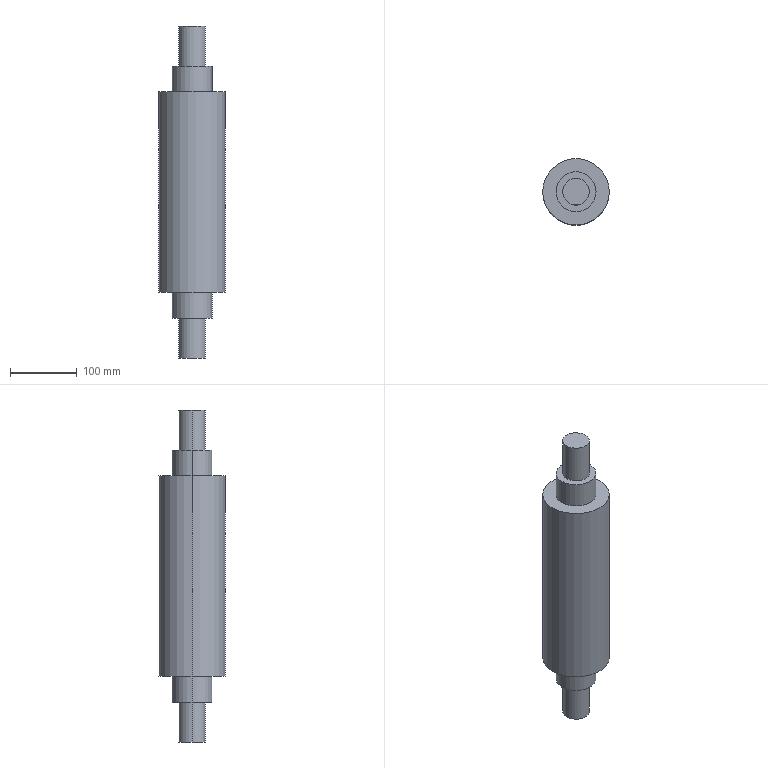Part | STEP file | 1 solid | 16 faces | box 100 x 100 x 498 mm | volume 2727531 mm3 | cylinder 10 | plane 6 | commonest cylinder face diameters 40 x4 60 x4 100 x2
STEP:
#1=CARTESIAN_POINT('',(0.,0.,0.));
#2=DIRECTION('',(0.,0.,1.));
#3=DIRECTION('',(1.,0.,0.));
#4=AXIS2_PLACEMENT_3D('',#1,#2,#3);
#5=CARTESIAN_POINT('',(20.,0.,438.));
#6=VERTEX_POINT('',#5);
#7=CARTESIAN_POINT('',(-20.,0.,438.));
#8=VERTEX_POINT('',#7);
#9=CARTESIAN_POINT('',(0.,0.,438.));
#10=DIRECTION('',(0.,0.,1.));
#11=DIRECTION('',(1.,0.,0.));
#12=AXIS2_PLACEMENT_3D('',#9,#10,#11);
#13=CIRCLE('',#12,20.);
#14=CARTESIAN_POINT('',(0.,0.,438.));
#15=DIRECTION('',(0.,0.,-1.));
#16=DIRECTION('',(-1.,0.,0.));
#17=AXIS2_PLACEMENT_3D('',#14,#15,#16);
#18=CYLINDRICAL_SURFACE('',#17,20.);
#19=CARTESIAN_POINT('',(3.142,0.));
#20=DIRECTION('',(-1.,0.));
#21=VECTOR('',#20,1.);
#22=LINE('',#19,#21);
#23=(GEOMETRIC_REPRESENTATION_CONTEXT(2)PARAMETRIC_REPRESENTATION_CONTEXT()REPRESENTATION_CONTEXT('',''));
#24=DEFINITIONAL_REPRESENTATION('',(#22),#23);
#25=PCURVE('',#18,#24);
#26=CARTESIAN_POINT('',(0.,0.,438.));
#27=DIRECTION('',(0.,0.,1.));
#28=DIRECTION('',(1.,0.,0.));
#29=AXIS2_PLACEMENT_3D('',#26,#27,#28);
#30=PLANE('',#29);
#31=CARTESIAN_POINT('',(0.,0.));
#32=DIRECTION('',(1.,0.));
#33=AXIS2_PLACEMENT_2D('',#31,#32);
#34=CIRCLE('',#33,20.);
#35=(GEOMETRIC_REPRESENTATION_CONTEXT(2)PARAMETRIC_REPRESENTATION_CONTEXT()REPRESENTATION_CONTEXT('',''));
#36=DEFINITIONAL_REPRESENTATION('',(#34),#35);
#37=PCURVE('',#30,#36);
#38=SURFACE_CURVE('',#13,(#25,#37),.PCURVE_S1.);
#39=EDGE_CURVE('',#6,#8,#38,.T.);
#40=ORIENTED_EDGE('',*,*,#39,.F.);
#41=CARTESIAN_POINT('',(20.,0.,378.));
#42=VERTEX_POINT('',#41);
#43=CARTESIAN_POINT('',(20.,0.,438.));
#44=DIRECTION('',(0.,0.,-1.));
#45=VECTOR('',#44,1.);
#46=LINE('',#43,#45);
#47=CARTESIAN_POINT('',(3.142,0.));
#48=DIRECTION('',(0.,1.));
#49=VECTOR('',#48,1.);
#50=LINE('',#47,#49);
#51=(GEOMETRIC_REPRESENTATION_CONTEXT(2)PARAMETRIC_REPRESENTATION_CONTEXT()REPRESENTATION_CONTEXT('',''));
#52=DEFINITIONAL_REPRESENTATION('',(#50),#51);
#53=PCURVE('',#18,#52);
#54=CARTESIAN_POINT('',(0.,0.,438.));
#55=DIRECTION('',(0.,0.,-1.));
#56=DIRECTION('',(-1.,0.,0.));
#57=AXIS2_PLACEMENT_3D('',#54,#55,#56);
#58=CYLINDRICAL_SURFACE('',#57,20.);
#59=CARTESIAN_POINT('',(3.142,0.));
#60=DIRECTION('',(0.,1.));
#61=VECTOR('',#60,1.);
#62=LINE('',#59,#61);
#63=(GEOMETRIC_REPRESENTATION_CONTEXT(2)PARAMETRIC_REPRESENTATION_CONTEXT()REPRESENTATION_CONTEXT('',''));
#64=DEFINITIONAL_REPRESENTATION('',(#62),#63);
#65=PCURVE('',#58,#64);
#66=SURFACE_CURVE('',#46,(#53,#65),.PCURVE_S1.);
#67=EDGE_CURVE('',#6,#42,#66,.T.);
#68=ORIENTED_EDGE('',*,*,#67,.T.);
#69=CARTESIAN_POINT('',(-20.,0.,378.));
#70=VERTEX_POINT('',#69);
#71=CARTESIAN_POINT('',(0.,0.,378.));
#72=DIRECTION('',(0.,0.,1.));
#73=DIRECTION('',(1.,0.,0.));
#74=AXIS2_PLACEMENT_3D('',#71,#72,#73);
#75=CIRCLE('',#74,20.);
#76=CARTESIAN_POINT('',(3.142,60.));
#77=DIRECTION('',(-1.,0.));
#78=VECTOR('',#77,1.);
#79=LINE('',#76,#78);
#80=(GEOMETRIC_REPRESENTATION_CONTEXT(2)PARAMETRIC_REPRESENTATION_CONTEXT()REPRESENTATION_CONTEXT('',''));
#81=DEFINITIONAL_REPRESENTATION('',(#79),#80);
#82=PCURVE('',#18,#81);
#83=CARTESIAN_POINT('',(0.,0.,378.));
#84=DIRECTION('',(0.,0.,1.));
#85=DIRECTION('',(1.,0.,0.));
#86=AXIS2_PLACEMENT_3D('',#83,#84,#85);
#87=PLANE('',#86);
#88=CARTESIAN_POINT('',(0.,0.));
#89=DIRECTION('',(1.,0.));
#90=AXIS2_PLACEMENT_2D('',#88,#89);
#91=CIRCLE('',#90,20.);
#92=(GEOMETRIC_REPRESENTATION_CONTEXT(2)PARAMETRIC_REPRESENTATION_CONTEXT()REPRESENTATION_CONTEXT('',''));
#93=DEFINITIONAL_REPRESENTATION('',(#91),#92);
#94=PCURVE('',#87,#93);
#95=SURFACE_CURVE('',#75,(#82,#94),.PCURVE_S1.);
#96=EDGE_CURVE('',#42,#70,#95,.T.);
#97=ORIENTED_EDGE('',*,*,#96,.T.);
#98=CARTESIAN_POINT('',(-20.,0.,438.));
#99=DIRECTION('',(0.,0.,-1.));
#100=VECTOR('',#99,1.);
#101=LINE('',#98,#100);
#102=CARTESIAN_POINT('',(0.,0.));
#103=DIRECTION('',(0.,1.));
#104=VECTOR('',#103,1.);
#105=LINE('',#102,#104);
#106=(GEOMETRIC_REPRESENTATION_CONTEXT(2)PARAMETRIC_REPRESENTATION_CONTEXT()REPRESENTATION_CONTEXT('',''));
#107=DEFINITIONAL_REPRESENTATION('',(#105),#106);
#108=PCURVE('',#18,#107);
#109=CARTESIAN_POINT('',(6.283,0.));
#110=DIRECTION('',(0.,1.));
#111=VECTOR('',#110,1.);
#112=LINE('',#109,#111);
#113=(GEOMETRIC_REPRESENTATION_CONTEXT(2)PARAMETRIC_REPRESENTATION_CONTEXT()REPRESENTATION_CONTEXT('',''));
#114=DEFINITIONAL_REPRESENTATION('',(#112),#113);
#115=PCURVE('',#58,#114);
#116=SURFACE_CURVE('',#101,(#108,#115),.PCURVE_S1.);
#117=EDGE_CURVE('',#8,#70,#116,.T.);
#118=ORIENTED_EDGE('',*,*,#117,.F.);
#119=EDGE_LOOP('',(#40,#68,#97,#118));
#120=FACE_BOUND('',#119,.T.);
#121=ADVANCED_FACE('',(#120),#18,.T.);
#122=CARTESIAN_POINT('',(30.,0.,378.));
#123=VERTEX_POINT('',#122);
#124=CARTESIAN_POINT('',(-30.,0.,378.));
#125=VERTEX_POINT('',#124);
#126=CARTESIAN_POINT('',(0.,0.,378.));
#127=DIRECTION('',(0.,0.,1.));
#128=DIRECTION('',(1.,0.,0.));
#129=AXIS2_PLACEMENT_3D('',#126,#127,#128);
#130=CIRCLE('',#129,30.);
#131=CARTESIAN_POINT('',(0.,0.,378.));
#132=DIRECTION('',(0.,0.,-1.));
#133=DIRECTION('',(-1.,0.,0.));
#134=AXIS2_PLACEMENT_3D('',#131,#132,#133);
#135=CYLINDRICAL_SURFACE('',#134,30.);
#136=CARTESIAN_POINT('',(3.142,0.));
#137=DIRECTION('',(-1.,0.));
#138=VECTOR('',#137,1.);
#139=LINE('',#136,#138);
#140=(GEOMETRIC_REPRESENTATION_CONTEXT(2)PARAMETRIC_REPRESENTATION_CONTEXT()REPRESENTATION_CONTEXT('',''));
#141=DEFINITIONAL_REPRESENTATION('',(#139),#140);
#142=PCURVE('',#135,#141);
#143=CARTESIAN_POINT('',(0.,0.));
#144=DIRECTION('',(1.,0.));
#145=AXIS2_PLACEMENT_2D('',#143,#144);
#146=CIRCLE('',#145,30.);
#147=(GEOMETRIC_REPRESENTATION_CONTEXT(2)PARAMETRIC_REPRESENTATION_CONTEXT()REPRESENTATION_CONTEXT('',''));
#148=DEFINITIONAL_REPRESENTATION('',(#146),#147);
#149=PCURVE('',#87,#148);
#150=SURFACE_CURVE('',#130,(#142,#149),.PCURVE_S1.);
#151=EDGE_CURVE('',#123,#125,#150,.T.);
#152=ORIENTED_EDGE('',*,*,#151,.F.);
#153=CARTESIAN_POINT('',(30.,0.,339.));
#154=VERTEX_POINT('',#153);
#155=CARTESIAN_POINT('',(30.,0.,378.));
#156=DIRECTION('',(0.,0.,-1.));
#157=VECTOR('',#156,1.);
#158=LINE('',#155,#157);
#159=CARTESIAN_POINT('',(3.142,0.));
#160=DIRECTION('',(0.,1.));
#161=VECTOR('',#160,1.);
#162=LINE('',#159,#161);
#163=(GEOMETRIC_REPRESENTATION_CONTEXT(2)PARAMETRIC_REPRESENTATION_CONTEXT()REPRESENTATION_CONTEXT('',''));
#164=DEFINITIONAL_REPRESENTATION('',(#162),#163);
#165=PCURVE('',#135,#164);
#166=CARTESIAN_POINT('',(0.,0.,378.));
#167=DIRECTION('',(0.,0.,-1.));
#168=DIRECTION('',(-1.,0.,0.));
#169=AXIS2_PLACEMENT_3D('',#166,#167,#168);
#170=CYLINDRICAL_SURFACE('',#169,30.);
#171=CARTESIAN_POINT('',(3.142,0.));
#172=DIRECTION('',(0.,1.));
#173=VECTOR('',#172,1.);
#174=LINE('',#171,#173);
#175=(GEOMETRIC_REPRESENTATION_CONTEXT(2)PARAMETRIC_REPRESENTATION_CONTEXT()REPRESENTATION_CONTEXT('',''));
#176=DEFINITIONAL_REPRESENTATION('',(#174),#175);
#177=PCURVE('',#170,#176);
#178=SURFACE_CURVE('',#158,(#165,#177),.PCURVE_S1.);
#179=EDGE_CURVE('',#123,#154,#178,.T.);
#180=ORIENTED_EDGE('',*,*,#179,.T.);
#181=CARTESIAN_POINT('',(-30.,0.,339.));
#182=VERTEX_POINT('',#181);
#183=CARTESIAN_POINT('',(0.,0.,339.));
#184=DIRECTION('',(0.,0.,1.));
#185=DIRECTION('',(1.,0.,0.));
#186=AXIS2_PLACEMENT_3D('',#183,#184,#185);
#187=CIRCLE('',#186,30.);
#188=CARTESIAN_POINT('',(3.142,39.));
#189=DIRECTION('',(-1.,0.));
#190=VECTOR('',#189,1.);
#191=LINE('',#188,#190);
#192=(GEOMETRIC_REPRESENTATION_CONTEXT(2)PARAMETRIC_REPRESENTATION_CONTEXT()REPRESENTATION_CONTEXT('',''));
#193=DEFINITIONAL_REPRESENTATION('',(#191),#192);
#194=PCURVE('',#135,#193);
#195=CARTESIAN_POINT('',(0.,0.,339.));
#196=DIRECTION('',(0.,0.,1.));
#197=DIRECTION('',(1.,0.,0.));
#198=AXIS2_PLACEMENT_3D('',#195,#196,#197);
#199=PLANE('',#198);
#200=CARTESIAN_POINT('',(0.,0.));
#201=DIRECTION('',(1.,0.));
#202=AXIS2_PLACEMENT_2D('',#200,#201);
#203=CIRCLE('',#202,30.);
#204=(GEOMETRIC_REPRESENTATION_CONTEXT(2)PARAMETRIC_REPRESENTATION_CONTEXT()REPRESENTATION_CONTEXT('',''));
#205=DEFINITIONAL_REPRESENTATION('',(#203),#204);
#206=PCURVE('',#199,#205);
#207=SURFACE_CURVE('',#187,(#194,#206),.PCURVE_S1.);
#208=EDGE_CURVE('',#154,#182,#207,.T.);
#209=ORIENTED_EDGE('',*,*,#208,.T.);
#210=CARTESIAN_POINT('',(-30.,0.,378.));
#211=DIRECTION('',(0.,0.,-1.));
#212=VECTOR('',#211,1.);
#213=LINE('',#210,#212);
#214=CARTESIAN_POINT('',(0.,0.));
#215=DIRECTION('',(0.,1.));
#216=VECTOR('',#215,1.);
#217=LINE('',#214,#216);
#218=(GEOMETRIC_REPRESENTATION_CONTEXT(2)PARAMETRIC_REPRESENTATION_CONTEXT()REPRESENTATION_CONTEXT('',''));
#219=DEFINITIONAL_REPRESENTATION('',(#217),#218);
#220=PCURVE('',#135,#219);
#221=CARTESIAN_POINT('',(6.283,0.));
#222=DIRECTION('',(0.,1.));
#223=VECTOR('',#222,1.);
#224=LINE('',#221,#223);
#225=(GEOMETRIC_REPRESENTATION_CONTEXT(2)PARAMETRIC_REPRESENTATION_CONTEXT()REPRESENTATION_CONTEXT('',''));
#226=DEFINITIONAL_REPRESENTATION('',(#224),#225);
#227=PCURVE('',#170,#226);
#228=SURFACE_CURVE('',#213,(#220,#227),.PCURVE_S1.);
#229=EDGE_CURVE('',#125,#182,#228,.T.);
#230=ORIENTED_EDGE('',*,*,#229,.F.);
#231=EDGE_LOOP('',(#152,#180,#209,#230));
#232=FACE_BOUND('',#231,.T.);
#233=ADVANCED_FACE('',(#232),#135,.T.);
#234=CARTESIAN_POINT('',(-20.,0.,-60.));
#235=VERTEX_POINT('',#234);
#236=CARTESIAN_POINT('',(20.,0.,-60.));
#237=VERTEX_POINT('',#236);
#238=CARTESIAN_POINT('',(0.,0.,-60.));
#239=DIRECTION('',(0.,0.,-1.));
#240=DIRECTION('',(-1.,0.,0.));
#241=AXIS2_PLACEMENT_3D('',#238,#239,#240);
#242=CIRCLE('',#241,20.);
#243=CARTESIAN_POINT('',(0.,0.,-60.));
#244=DIRECTION('',(0.,0.,1.));
#245=DIRECTION('',(1.,0.,0.));
#246=AXIS2_PLACEMENT_3D('',#243,#244,#245);
#247=CYLINDRICAL_SURFACE('',#246,20.);
#248=CARTESIAN_POINT('',(3.142,0.));
#249=DIRECTION('',(-1.,0.));
#250=VECTOR('',#249,1.);
#251=LINE('',#248,#250);
#252=(GEOMETRIC_REPRESENTATION_CONTEXT(2)PARAMETRIC_REPRESENTATION_CONTEXT()REPRESENTATION_CONTEXT('',''));
#253=DEFINITIONAL_REPRESENTATION('',(#251),#252);
#254=PCURVE('',#247,#253);
#255=CARTESIAN_POINT('',(0.,0.,-60.));
#256=DIRECTION('',(0.,0.,-1.));
#257=DIRECTION('',(-1.,0.,0.));
#258=AXIS2_PLACEMENT_3D('',#255,#256,#257);
#259=PLANE('',#258);
#260=CARTESIAN_POINT('',(0.,0.));
#261=DIRECTION('',(1.,0.));
#262=AXIS2_PLACEMENT_2D('',#260,#261);
#263=CIRCLE('',#262,20.);
#264=(GEOMETRIC_REPRESENTATION_CONTEXT(2)PARAMETRIC_REPRESENTATION_CONTEXT()REPRESENTATION_CONTEXT('',''));
#265=DEFINITIONAL_REPRESENTATION('',(#263),#264);
#266=PCURVE('',#259,#265);
#267=SURFACE_CURVE('',#242,(#254,#266),.PCURVE_S1.);
#268=EDGE_CURVE('',#235,#237,#267,.T.);
#269=ORIENTED_EDGE('',*,*,#268,.F.);
#270=CARTESIAN_POINT('',(-20.,0.,0.));
#271=VERTEX_POINT('',#270);
#272=CARTESIAN_POINT('',(-20.,0.,-60.));
#273=DIRECTION('',(0.,0.,1.));
#274=VECTOR('',#273,1.);
#275=LINE('',#272,#274);
#276=CARTESIAN_POINT('',(3.142,0.));
#277=DIRECTION('',(0.,1.));
#278=VECTOR('',#277,1.);
#279=LINE('',#276,#278);
#280=(GEOMETRIC_REPRESENTATION_CONTEXT(2)PARAMETRIC_REPRESENTATION_CONTEXT()REPRESENTATION_CONTEXT('',''));
#281=DEFINITIONAL_REPRESENTATION('',(#279),#280);
#282=PCURVE('',#247,#281);
#283=CARTESIAN_POINT('',(0.,0.,-60.));
#284=DIRECTION('',(0.,0.,1.));
#285=DIRECTION('',(1.,0.,0.));
#286=AXIS2_PLACEMENT_3D('',#283,#284,#285);
#287=CYLINDRICAL_SURFACE('',#286,20.);
#288=CARTESIAN_POINT('',(3.142,0.));
#289=DIRECTION('',(0.,1.));
#290=VECTOR('',#289,1.);
#291=LINE('',#288,#290);
#292=(GEOMETRIC_REPRESENTATION_CONTEXT(2)PARAMETRIC_REPRESENTATION_CONTEXT()REPRESENTATION_CONTEXT('',''));
#293=DEFINITIONAL_REPRESENTATION('',(#291),#292);
#294=PCURVE('',#287,#293);
#295=SURFACE_CURVE('',#275,(#282,#294),.PCURVE_S1.);
#296=EDGE_CURVE('',#235,#271,#295,.T.);
#297=ORIENTED_EDGE('',*,*,#296,.T.);
#298=CARTESIAN_POINT('',(20.,0.,0.));
#299=VERTEX_POINT('',#298);
#300=CARTESIAN_POINT('',(0.,0.,0.));
#301=DIRECTION('',(0.,0.,-1.));
#302=DIRECTION('',(-1.,0.,0.));
#303=AXIS2_PLACEMENT_3D('',#300,#301,#302);
#304=CIRCLE('',#303,20.);
#305=CARTESIAN_POINT('',(3.142,60.));
#306=DIRECTION('',(-1.,0.));
#307=VECTOR('',#306,1.);
#308=LINE('',#305,#307);
#309=(GEOMETRIC_REPRESENTATION_CONTEXT(2)PARAMETRIC_REPRESENTATION_CONTEXT()REPRESENTATION_CONTEXT('',''));
#310=DEFINITIONAL_REPRESENTATION('',(#308),#309);
#311=PCURVE('',#247,#310);
#312=CARTESIAN_POINT('',(0.,0.,0.));
#313=DIRECTION('',(0.,0.,1.));
#314=DIRECTION('',(1.,0.,0.));
#315=AXIS2_PLACEMENT_3D('',#312,#313,#314);
#316=PLANE('',#315);
#317=CARTESIAN_POINT('',(-20.,0.));
#318=CARTESIAN_POINT('',(-20.,34.641));
#319=CARTESIAN_POINT('',(10.,17.321));
#320=CARTESIAN_POINT('',(40.,0.));
#321=CARTESIAN_POINT('',(10.,-17.321));
#322=CARTESIAN_POINT('',(-20.,-34.641));
#323=CARTESIAN_POINT('',(-20.,0.));
#324=(BOUNDED_CURVE()B_SPLINE_CURVE(2,(#317,#318,#319,#320,#321,#322,#323),.UNSPECIFIED.,.T.,.F.)B_SPLINE_CURVE_WITH_KNOTS((1,2,2,2,2,1),(-2.094,0.,2.094,4.189,6.283,8.378),.UNSPECIFIED.)CURVE()GEOMETRIC_REPRESENTATION_ITEM()RATIONAL_B_SPLINE_CURVE((1.,0.5,1.,0.5,1.,0.5,1.))REPRESENTATION_ITEM(''));
#325=(GEOMETRIC_REPRESENTATION_CONTEXT(2)PARAMETRIC_REPRESENTATION_CONTEXT()REPRESENTATION_CONTEXT('',''));
#326=DEFINITIONAL_REPRESENTATION('',(#324),#325);
#327=PCURVE('',#316,#326);
#328=SURFACE_CURVE('',#304,(#311,#327),.PCURVE_S1.);
#329=EDGE_CURVE('',#271,#299,#328,.T.);
#330=ORIENTED_EDGE('',*,*,#329,.T.);
#331=CARTESIAN_POINT('',(20.,0.,-60.));
#332=DIRECTION('',(0.,0.,1.));
#333=VECTOR('',#332,1.);
#334=LINE('',#331,#333);
#335=CARTESIAN_POINT('',(0.,0.));
#336=DIRECTION('',(0.,1.));
#337=VECTOR('',#336,1.);
#338=LINE('',#335,#337);
#339=(GEOMETRIC_REPRESENTATION_CONTEXT(2)PARAMETRIC_REPRESENTATION_CONTEXT()REPRESENTATION_CONTEXT('',''));
#340=DEFINITIONAL_REPRESENTATION('',(#338),#339);
#341=PCURVE('',#247,#340);
#342=CARTESIAN_POINT('',(6.283,0.));
#343=DIRECTION('',(0.,1.));
#344=VECTOR('',#343,1.);
#345=LINE('',#342,#344);
#346=(GEOMETRIC_REPRESENTATION_CONTEXT(2)PARAMETRIC_REPRESENTATION_CONTEXT()REPRESENTATION_CONTEXT('',''));
#347=DEFINITIONAL_REPRESENTATION('',(#345),#346);
#348=PCURVE('',#287,#347);
#349=SURFACE_CURVE('',#334,(#341,#348),.PCURVE_S1.);
#350=EDGE_CURVE('',#237,#299,#349,.T.);
#351=ORIENTED_EDGE('',*,*,#350,.F.);
#352=EDGE_LOOP('',(#269,#297,#330,#351));
#353=FACE_BOUND('',#352,.T.);
#354=ADVANCED_FACE('',(#353),#247,.T.);
#355=CARTESIAN_POINT('',(50.,0.,339.));
#356=VERTEX_POINT('',#355);
#357=CARTESIAN_POINT('',(-50.,0.,339.));
#358=VERTEX_POINT('',#357);
#359=CARTESIAN_POINT('',(0.,0.,339.));
#360=DIRECTION('',(0.,0.,1.));
#361=DIRECTION('',(1.,0.,0.));
#362=AXIS2_PLACEMENT_3D('',#359,#360,#361);
#363=CIRCLE('',#362,50.);
#364=CARTESIAN_POINT('',(0.,0.,339.));
#365=DIRECTION('',(0.,0.,-1.));
#366=DIRECTION('',(-1.,0.,0.));
#367=AXIS2_PLACEMENT_3D('',#364,#365,#366);
#368=CYLINDRICAL_SURFACE('',#367,50.);
#369=CARTESIAN_POINT('',(3.142,0.));
#370=DIRECTION('',(-1.,0.));
#371=VECTOR('',#370,1.);
#372=LINE('',#369,#371);
#373=(GEOMETRIC_REPRESENTATION_CONTEXT(2)PARAMETRIC_REPRESENTATION_CONTEXT()REPRESENTATION_CONTEXT('',''));
#374=DEFINITIONAL_REPRESENTATION('',(#372),#373);
#375=PCURVE('',#368,#374);
#376=CARTESIAN_POINT('',(0.,0.));
#377=DIRECTION('',(1.,0.));
#378=AXIS2_PLACEMENT_2D('',#376,#377);
#379=CIRCLE('',#378,50.);
#380=(GEOMETRIC_REPRESENTATION_CONTEXT(2)PARAMETRIC_REPRESENTATION_CONTEXT()REPRESENTATION_CONTEXT('',''));
#381=DEFINITIONAL_REPRESENTATION('',(#379),#380);
#382=PCURVE('',#199,#381);
#383=SURFACE_CURVE('',#363,(#375,#382),.PCURVE_S1.);
#384=EDGE_CURVE('',#356,#358,#383,.T.);
#385=ORIENTED_EDGE('',*,*,#384,.F.);
#386=CARTESIAN_POINT('',(50.,0.,39.));
#387=VERTEX_POINT('',#386);
#388=CARTESIAN_POINT('',(50.,0.,339.));
#389=DIRECTION('',(0.,0.,-1.));
#390=VECTOR('',#389,1.);
#391=LINE('',#388,#390);
#392=CARTESIAN_POINT('',(3.142,0.));
#393=DIRECTION('',(0.,1.));
#394=VECTOR('',#393,1.);
#395=LINE('',#392,#394);
#396=(GEOMETRIC_REPRESENTATION_CONTEXT(2)PARAMETRIC_REPRESENTATION_CONTEXT()REPRESENTATION_CONTEXT('',''));
#397=DEFINITIONAL_REPRESENTATION('',(#395),#396);
#398=PCURVE('',#368,#397);
#399=CARTESIAN_POINT('',(0.,0.,339.));
#400=DIRECTION('',(0.,0.,-1.));
#401=DIRECTION('',(-1.,0.,0.));
#402=AXIS2_PLACEMENT_3D('',#399,#400,#401);
#403=CYLINDRICAL_SURFACE('',#402,50.);
#404=CARTESIAN_POINT('',(3.142,0.));
#405=DIRECTION('',(0.,1.));
#406=VECTOR('',#405,1.);
#407=LINE('',#404,#406);
#408=(GEOMETRIC_REPRESENTATION_CONTEXT(2)PARAMETRIC_REPRESENTATION_CONTEXT()REPRESENTATION_CONTEXT('',''));
#409=DEFINITIONAL_REPRESENTATION('',(#407),#408);
#410=PCURVE('',#403,#409);
#411=SURFACE_CURVE('',#391,(#398,#410),.PCURVE_S1.);
#412=EDGE_CURVE('',#356,#387,#411,.T.);
#413=ORIENTED_EDGE('',*,*,#412,.T.);
#414=CARTESIAN_POINT('',(-50.,0.,39.));
#415=VERTEX_POINT('',#414);
#416=CARTESIAN_POINT('',(0.,0.,39.));
#417=DIRECTION('',(0.,0.,1.));
#418=DIRECTION('',(1.,0.,0.));
#419=AXIS2_PLACEMENT_3D('',#416,#417,#418);
#420=CIRCLE('',#419,50.);
#421=CARTESIAN_POINT('',(3.142,300.));
#422=DIRECTION('',(-1.,0.));
#423=VECTOR('',#422,1.);
#424=LINE('',#421,#423);
#425=(GEOMETRIC_REPRESENTATION_CONTEXT(2)PARAMETRIC_REPRESENTATION_CONTEXT()REPRESENTATION_CONTEXT('',''));
#426=DEFINITIONAL_REPRESENTATION('',(#424),#425);
#427=PCURVE('',#368,#426);
#428=CARTESIAN_POINT('',(0.,0.,39.));
#429=DIRECTION('',(0.,0.,1.));
#430=DIRECTION('',(1.,0.,0.));
#431=AXIS2_PLACEMENT_3D('',#428,#429,#430);
#432=PLANE('',#431);
#433=CARTESIAN_POINT('',(0.,0.));
#434=DIRECTION('',(1.,0.));
#435=AXIS2_PLACEMENT_2D('',#433,#434);
#436=CIRCLE('',#435,50.);
#437=(GEOMETRIC_REPRESENTATION_CONTEXT(2)PARAMETRIC_REPRESENTATION_CONTEXT()REPRESENTATION_CONTEXT('',''));
#438=DEFINITIONAL_REPRESENTATION('',(#436),#437);
#439=PCURVE('',#432,#438);
#440=SURFACE_CURVE('',#420,(#427,#439),.PCURVE_S1.);
#441=EDGE_CURVE('',#387,#415,#440,.T.);
#442=ORIENTED_EDGE('',*,*,#441,.T.);
#443=CARTESIAN_POINT('',(-50.,0.,339.));
#444=DIRECTION('',(0.,0.,-1.));
#445=VECTOR('',#444,1.);
#446=LINE('',#443,#445);
#447=CARTESIAN_POINT('',(0.,0.));
#448=DIRECTION('',(0.,1.));
#449=VECTOR('',#448,1.);
#450=LINE('',#447,#449);
#451=(GEOMETRIC_REPRESENTATION_CONTEXT(2)PARAMETRIC_REPRESENTATION_CONTEXT()REPRESENTATION_CONTEXT('',''));
#452=DEFINITIONAL_REPRESENTATION('',(#450),#451);
#453=PCURVE('',#368,#452);
#454=CARTESIAN_POINT('',(6.283,0.));
#455=DIRECTION('',(0.,1.));
#456=VECTOR('',#455,1.);
#457=LINE('',#454,#456);
#458=(GEOMETRIC_REPRESENTATION_CONTEXT(2)PARAMETRIC_REPRESENTATION_CONTEXT()REPRESENTATION_CONTEXT('',''));
#459=DEFINITIONAL_REPRESENTATION('',(#457),#458);
#460=PCURVE('',#403,#459);
#461=SURFACE_CURVE('',#446,(#453,#460),.PCURVE_S1.);
#462=EDGE_CURVE('',#358,#415,#461,.T.);
#463=ORIENTED_EDGE('',*,*,#462,.F.);
#464=EDGE_LOOP('',(#385,#413,#442,#463));
#465=FACE_BOUND('',#464,.T.);
#466=ADVANCED_FACE('',(#465),#368,.T.);
#467=CARTESIAN_POINT('',(30.,0.,39.));
#468=VERTEX_POINT('',#467);
#469=CARTESIAN_POINT('',(-30.,0.,39.));
#470=VERTEX_POINT('',#469);
#471=CARTESIAN_POINT('',(0.,0.,39.));
#472=DIRECTION('',(0.,0.,1.));
#473=DIRECTION('',(1.,0.,0.));
#474=AXIS2_PLACEMENT_3D('',#471,#472,#473);
#475=CIRCLE('',#474,30.);
#476=CARTESIAN_POINT('',(0.,0.,39.));
#477=DIRECTION('',(0.,0.,-1.));
#478=DIRECTION('',(-1.,0.,0.));
#479=AXIS2_PLACEMENT_3D('',#476,#477,#478);
#480=CYLINDRICAL_SURFACE('',#479,30.);
#481=CARTESIAN_POINT('',(3.142,0.));
#482=DIRECTION('',(-1.,0.));
#483=VECTOR('',#482,1.);
#484=LINE('',#481,#483);
#485=(GEOMETRIC_REPRESENTATION_CONTEXT(2)PARAMETRIC_REPRESENTATION_CONTEXT()REPRESENTATION_CONTEXT('',''));
#486=DEFINITIONAL_REPRESENTATION('',(#484),#485);
#487=PCURVE('',#480,#486);
#488=CARTESIAN_POINT('',(0.,0.));
#489=DIRECTION('',(1.,0.));
#490=AXIS2_PLACEMENT_2D('',#488,#489);
#491=CIRCLE('',#490,30.);
#492=(GEOMETRIC_REPRESENTATION_CONTEXT(2)PARAMETRIC_REPRESENTATION_CONTEXT()REPRESENTATION_CONTEXT('',''));
#493=DEFINITIONAL_REPRESENTATION('',(#491),#492);
#494=PCURVE('',#432,#493);
#495=SURFACE_CURVE('',#475,(#487,#494),.PCURVE_S1.);
#496=EDGE_CURVE('',#468,#470,#495,.T.);
#497=ORIENTED_EDGE('',*,*,#496,.F.);
#498=CARTESIAN_POINT('',(30.,0.,0.));
#499=VERTEX_POINT('',#498);
#500=CARTESIAN_POINT('',(30.,0.,39.));
#501=DIRECTION('',(0.,0.,-1.));
#502=VECTOR('',#501,1.);
#503=LINE('',#500,#502);
#504=CARTESIAN_POINT('',(3.142,0.));
#505=DIRECTION('',(0.,1.));
#506=VECTOR('',#505,1.);
#507=LINE('',#504,#506);
#508=(GEOMETRIC_REPRESENTATION_CONTEXT(2)PARAMETRIC_REPRESENTATION_CONTEXT()REPRESENTATION_CONTEXT('',''));
#509=DEFINITIONAL_REPRESENTATION('',(#507),#508);
#510=PCURVE('',#480,#509);
#511=CARTESIAN_POINT('',(0.,0.,39.));
#512=DIRECTION('',(0.,0.,-1.));
#513=DIRECTION('',(-1.,0.,0.));
#514=AXIS2_PLACEMENT_3D('',#511,#512,#513);
#515=CYLINDRICAL_SURFACE('',#514,30.);
#516=CARTESIAN_POINT('',(3.142,0.));
#517=DIRECTION('',(0.,1.));
#518=VECTOR('',#517,1.);
#519=LINE('',#516,#518);
#520=(GEOMETRIC_REPRESENTATION_CONTEXT(2)PARAMETRIC_REPRESENTATION_CONTEXT()REPRESENTATION_CONTEXT('',''));
#521=DEFINITIONAL_REPRESENTATION('',(#519),#520);
#522=PCURVE('',#515,#521);
#523=SURFACE_CURVE('',#503,(#510,#522),.PCURVE_S1.);
#524=EDGE_CURVE('',#468,#499,#523,.T.);
#525=ORIENTED_EDGE('',*,*,#524,.T.);
#526=CARTESIAN_POINT('',(-30.,0.,0.));
#527=VERTEX_POINT('',#526);
#528=CARTESIAN_POINT('',(0.,0.,0.));
#529=DIRECTION('',(0.,0.,1.));
#530=DIRECTION('',(1.,0.,0.));
#531=AXIS2_PLACEMENT_3D('',#528,#529,#530);
#532=CIRCLE('',#531,30.);
#533=CARTESIAN_POINT('',(3.142,39.));
#534=DIRECTION('',(-1.,0.));
#535=VECTOR('',#534,1.);
#536=LINE('',#533,#535);
#537=(GEOMETRIC_REPRESENTATION_CONTEXT(2)PARAMETRIC_REPRESENTATION_CONTEXT()REPRESENTATION_CONTEXT('',''));
#538=DEFINITIONAL_REPRESENTATION('',(#536),#537);
#539=PCURVE('',#480,#538);
#540=CARTESIAN_POINT('',(0.,0.));
#541=DIRECTION('',(1.,0.));
#542=AXIS2_PLACEMENT_2D('',#540,#541);
#543=CIRCLE('',#542,30.);
#544=(GEOMETRIC_REPRESENTATION_CONTEXT(2)PARAMETRIC_REPRESENTATION_CONTEXT()REPRESENTATION_CONTEXT('',''));
#545=DEFINITIONAL_REPRESENTATION('',(#543),#544);
#546=PCURVE('',#316,#545);
#547=SURFACE_CURVE('',#532,(#539,#546),.PCURVE_S1.);
#548=EDGE_CURVE('',#499,#527,#547,.T.);
#549=ORIENTED_EDGE('',*,*,#548,.T.);
#550=CARTESIAN_POINT('',(-30.,0.,39.));
#551=DIRECTION('',(0.,0.,-1.));
#552=VECTOR('',#551,1.);
#553=LINE('',#550,#552);
#554=CARTESIAN_POINT('',(0.,0.));
#555=DIRECTION('',(0.,1.));
#556=VECTOR('',#555,1.);
#557=LINE('',#554,#556);
#558=(GEOMETRIC_REPRESENTATION_CONTEXT(2)PARAMETRIC_REPRESENTATION_CONTEXT()REPRESENTATION_CONTEXT('',''));
#559=DEFINITIONAL_REPRESENTATION('',(#557),#558);
#560=PCURVE('',#480,#559);
#561=CARTESIAN_POINT('',(6.283,0.));
#562=DIRECTION('',(0.,1.));
#563=VECTOR('',#562,1.);
#564=LINE('',#561,#563);
#565=(GEOMETRIC_REPRESENTATION_CONTEXT(2)PARAMETRIC_REPRESENTATION_CONTEXT()REPRESENTATION_CONTEXT('',''));
#566=DEFINITIONAL_REPRESENTATION('',(#564),#565);
#567=PCURVE('',#515,#566);
#568=SURFACE_CURVE('',#553,(#560,#567),.PCURVE_S1.);
#569=EDGE_CURVE('',#470,#527,#568,.T.);
#570=ORIENTED_EDGE('',*,*,#569,.F.);
#571=EDGE_LOOP('',(#497,#525,#549,#570));
#572=FACE_BOUND('',#571,.T.);
#573=ADVANCED_FACE('',(#572),#480,.T.);
#574=ORIENTED_EDGE('',*,*,#524,.F.);
#575=CARTESIAN_POINT('',(0.,0.,39.));
#576=DIRECTION('',(0.,0.,1.));
#577=DIRECTION('',(1.,0.,0.));
#578=AXIS2_PLACEMENT_3D('',#575,#576,#577);
#579=CIRCLE('',#578,30.);
#580=CARTESIAN_POINT('',(9.425,0.));
#581=DIRECTION('',(-1.,0.));
#582=VECTOR('',#581,1.);
#583=LINE('',#580,#582);
#584=(GEOMETRIC_REPRESENTATION_CONTEXT(2)PARAMETRIC_REPRESENTATION_CONTEXT()REPRESENTATION_CONTEXT('',''));
#585=DEFINITIONAL_REPRESENTATION('',(#583),#584);
#586=PCURVE('',#515,#585);
#587=CARTESIAN_POINT('',(0.,0.));
#588=DIRECTION('',(1.,0.));
#589=AXIS2_PLACEMENT_2D('',#587,#588);
#590=CIRCLE('',#589,30.);
#591=(GEOMETRIC_REPRESENTATION_CONTEXT(2)PARAMETRIC_REPRESENTATION_CONTEXT()REPRESENTATION_CONTEXT('',''));
#592=DEFINITIONAL_REPRESENTATION('',(#590),#591);
#593=PCURVE('',#432,#592);
#594=SURFACE_CURVE('',#579,(#586,#593),.PCURVE_S1.);
#595=EDGE_CURVE('',#470,#468,#594,.T.);
#596=ORIENTED_EDGE('',*,*,#595,.F.);
#597=ORIENTED_EDGE('',*,*,#569,.T.);
#598=CARTESIAN_POINT('',(0.,0.,0.));
#599=DIRECTION('',(0.,0.,1.));
#600=DIRECTION('',(1.,0.,0.));
#601=AXIS2_PLACEMENT_3D('',#598,#599,#600);
#602=CIRCLE('',#601,30.);
#603=CARTESIAN_POINT('',(9.425,39.));
#604=DIRECTION('',(-1.,0.));
#605=VECTOR('',#604,1.);
#606=LINE('',#603,#605);
#607=(GEOMETRIC_REPRESENTATION_CONTEXT(2)PARAMETRIC_REPRESENTATION_CONTEXT()REPRESENTATION_CONTEXT('',''));
#608=DEFINITIONAL_REPRESENTATION('',(#606),#607);
#609=PCURVE('',#515,#608);
#610=CARTESIAN_POINT('',(0.,0.));
#611=DIRECTION('',(1.,0.));
#612=AXIS2_PLACEMENT_2D('',#610,#611);
#613=CIRCLE('',#612,30.);
#614=(GEOMETRIC_REPRESENTATION_CONTEXT(2)PARAMETRIC_REPRESENTATION_CONTEXT()REPRESENTATION_CONTEXT('',''));
#615=DEFINITIONAL_REPRESENTATION('',(#613),#614);
#616=PCURVE('',#316,#615);
#617=SURFACE_CURVE('',#602,(#609,#616),.PCURVE_S1.);
#618=EDGE_CURVE('',#527,#499,#617,.T.);
#619=ORIENTED_EDGE('',*,*,#618,.T.);
#620=EDGE_LOOP('',(#574,#596,#597,#619));
#621=FACE_BOUND('',#620,.T.);
#622=ADVANCED_FACE('',(#621),#515,.T.);
#623=CARTESIAN_POINT('',(0.,0.,0.));
#624=DIRECTION('',(0.,0.,-1.));
#625=DIRECTION('',(-1.,0.,0.));
#626=AXIS2_PLACEMENT_3D('',#623,#624,#625);
#627=CIRCLE('',#626,20.);
#628=CARTESIAN_POINT('',(-20.,0.));
#629=CARTESIAN_POINT('',(-20.,34.641));
#630=CARTESIAN_POINT('',(10.,17.321));
#631=CARTESIAN_POINT('',(40.,0.));
#632=CARTESIAN_POINT('',(10.,-17.321));
#633=CARTESIAN_POINT('',(-20.,-34.641));
#634=CARTESIAN_POINT('',(-20.,0.));
#635=(BOUNDED_CURVE()B_SPLINE_CURVE(2,(#628,#629,#630,#631,#632,#633,#634),.UNSPECIFIED.,.T.,.F.)B_SPLINE_CURVE_WITH_KNOTS((1,2,2,2,2,1),(-2.094,0.,2.094,4.189,6.283,8.378),.UNSPECIFIED.)CURVE()GEOMETRIC_REPRESENTATION_ITEM()RATIONAL_B_SPLINE_CURVE((1.,0.5,1.,0.5,1.,0.5,1.))REPRESENTATION_ITEM(''));
#636=(GEOMETRIC_REPRESENTATION_CONTEXT(2)PARAMETRIC_REPRESENTATION_CONTEXT()REPRESENTATION_CONTEXT('',''));
#637=DEFINITIONAL_REPRESENTATION('',(#635),#636);
#638=PCURVE('',#316,#637);
#639=CARTESIAN_POINT('',(9.425,60.));
#640=DIRECTION('',(-1.,0.));
#641=VECTOR('',#640,1.);
#642=LINE('',#639,#641);
#643=(GEOMETRIC_REPRESENTATION_CONTEXT(2)PARAMETRIC_REPRESENTATION_CONTEXT()REPRESENTATION_CONTEXT('',''));
#644=DEFINITIONAL_REPRESENTATION('',(#642),#643);
#645=PCURVE('',#287,#644);
#646=SURFACE_CURVE('',#627,(#638,#645),.PCURVE_S1.);
#647=EDGE_CURVE('',#299,#271,#646,.T.);
#648=ORIENTED_EDGE('',*,*,#647,.F.);
#649=ORIENTED_EDGE('',*,*,#329,.F.);
#650=EDGE_LOOP('',(#648,#649));
#651=FACE_BOUND('',#650,.T.);
#652=ORIENTED_EDGE('',*,*,#618,.F.);
#653=ORIENTED_EDGE('',*,*,#548,.F.);
#654=EDGE_LOOP('',(#652,#653));
#655=FACE_BOUND('',#654,.T.);
#656=ADVANCED_FACE('',(#651,#655),#316,.F.);
#657=ORIENTED_EDGE('',*,*,#412,.F.);
#658=CARTESIAN_POINT('',(0.,0.,339.));
#659=DIRECTION('',(0.,0.,1.));
#660=DIRECTION('',(1.,0.,0.));
#661=AXIS2_PLACEMENT_3D('',#658,#659,#660);
#662=CIRCLE('',#661,50.);
#663=CARTESIAN_POINT('',(9.425,0.));
#664=DIRECTION('',(-1.,0.));
#665=VECTOR('',#664,1.);
#666=LINE('',#663,#665);
#667=(GEOMETRIC_REPRESENTATION_CONTEXT(2)PARAMETRIC_REPRESENTATION_CONTEXT()REPRESENTATION_CONTEXT('',''));
#668=DEFINITIONAL_REPRESENTATION('',(#666),#667);
#669=PCURVE('',#403,#668);
#670=CARTESIAN_POINT('',(0.,0.));
#671=DIRECTION('',(1.,0.));
#672=AXIS2_PLACEMENT_2D('',#670,#671);
#673=CIRCLE('',#672,50.);
#674=(GEOMETRIC_REPRESENTATION_CONTEXT(2)PARAMETRIC_REPRESENTATION_CONTEXT()REPRESENTATION_CONTEXT('',''));
#675=DEFINITIONAL_REPRESENTATION('',(#673),#674);
#676=PCURVE('',#199,#675);
#677=SURFACE_CURVE('',#662,(#669,#676),.PCURVE_S1.);
#678=EDGE_CURVE('',#358,#356,#677,.T.);
#679=ORIENTED_EDGE('',*,*,#678,.F.);
#680=ORIENTED_EDGE('',*,*,#462,.T.);
#681=CARTESIAN_POINT('',(0.,0.,39.));
#682=DIRECTION('',(0.,0.,1.));
#683=DIRECTION('',(1.,0.,0.));
#684=AXIS2_PLACEMENT_3D('',#681,#682,#683);
#685=CIRCLE('',#684,50.);
#686=CARTESIAN_POINT('',(9.425,300.));
#687=DIRECTION('',(-1.,0.));
#688=VECTOR('',#687,1.);
#689=LINE('',#686,#688);
#690=(GEOMETRIC_REPRESENTATION_CONTEXT(2)PARAMETRIC_REPRESENTATION_CONTEXT()REPRESENTATION_CONTEXT('',''));
#691=DEFINITIONAL_REPRESENTATION('',(#689),#690);
#692=PCURVE('',#403,#691);
#693=CARTESIAN_POINT('',(0.,0.));
#694=DIRECTION('',(1.,0.));
#695=AXIS2_PLACEMENT_2D('',#693,#694);
#696=CIRCLE('',#695,50.);
#697=(GEOMETRIC_REPRESENTATION_CONTEXT(2)PARAMETRIC_REPRESENTATION_CONTEXT()REPRESENTATION_CONTEXT('',''));
#698=DEFINITIONAL_REPRESENTATION('',(#696),#697);
#699=PCURVE('',#432,#698);
#700=SURFACE_CURVE('',#685,(#692,#699),.PCURVE_S1.);
#701=EDGE_CURVE('',#415,#387,#700,.T.);
#702=ORIENTED_EDGE('',*,*,#701,.T.);
#703=EDGE_LOOP('',(#657,#679,#680,#702));
#704=FACE_BOUND('',#703,.T.);
#705=ADVANCED_FACE('',(#704),#403,.T.);
#706=CARTESIAN_POINT('',(0.,0.,339.));
#707=DIRECTION('',(0.,0.,1.));
#708=DIRECTION('',(1.,0.,0.));
#709=AXIS2_PLACEMENT_3D('',#706,#707,#708);
#710=CIRCLE('',#709,30.);
#711=CARTESIAN_POINT('',(0.,0.));
#712=DIRECTION('',(1.,0.));
#713=AXIS2_PLACEMENT_2D('',#711,#712);
#714=CIRCLE('',#713,30.);
#715=(GEOMETRIC_REPRESENTATION_CONTEXT(2)PARAMETRIC_REPRESENTATION_CONTEXT()REPRESENTATION_CONTEXT('',''));
#716=DEFINITIONAL_REPRESENTATION('',(#714),#715);
#717=PCURVE('',#199,#716);
#718=CARTESIAN_POINT('',(9.425,39.));
#719=DIRECTION('',(-1.,0.));
#720=VECTOR('',#719,1.);
#721=LINE('',#718,#720);
#722=(GEOMETRIC_REPRESENTATION_CONTEXT(2)PARAMETRIC_REPRESENTATION_CONTEXT()REPRESENTATION_CONTEXT('',''));
#723=DEFINITIONAL_REPRESENTATION('',(#721),#722);
#724=PCURVE('',#170,#723);
#725=SURFACE_CURVE('',#710,(#717,#724),.PCURVE_S1.);
#726=EDGE_CURVE('',#182,#154,#725,.T.);
#727=ORIENTED_EDGE('',*,*,#726,.F.);
#728=ORIENTED_EDGE('',*,*,#208,.F.);
#729=EDGE_LOOP('',(#727,#728));
#730=FACE_BOUND('',#729,.T.);
#731=ORIENTED_EDGE('',*,*,#678,.T.);
#732=ORIENTED_EDGE('',*,*,#384,.T.);
#733=EDGE_LOOP('',(#731,#732));
#734=FACE_BOUND('',#733,.T.);
#735=ADVANCED_FACE('',(#730,#734),#199,.T.);
#736=ORIENTED_EDGE('',*,*,#595,.T.);
#737=ORIENTED_EDGE('',*,*,#496,.T.);
#738=EDGE_LOOP('',(#736,#737));
#739=FACE_BOUND('',#738,.T.);
#740=ORIENTED_EDGE('',*,*,#701,.F.);
#741=ORIENTED_EDGE('',*,*,#441,.F.);
#742=EDGE_LOOP('',(#740,#741));
#743=FACE_BOUND('',#742,.T.);
#744=ADVANCED_FACE('',(#739,#743),#432,.F.);
#745=ORIENTED_EDGE('',*,*,#296,.F.);
#746=CARTESIAN_POINT('',(0.,0.,-60.));
#747=DIRECTION('',(0.,0.,-1.));
#748=DIRECTION('',(-1.,0.,0.));
#749=AXIS2_PLACEMENT_3D('',#746,#747,#748);
#750=CIRCLE('',#749,20.);
#751=CARTESIAN_POINT('',(9.425,0.));
#752=DIRECTION('',(-1.,0.));
#753=VECTOR('',#752,1.);
#754=LINE('',#751,#753);
#755=(GEOMETRIC_REPRESENTATION_CONTEXT(2)PARAMETRIC_REPRESENTATION_CONTEXT()REPRESENTATION_CONTEXT('',''));
#756=DEFINITIONAL_REPRESENTATION('',(#754),#755);
#757=PCURVE('',#287,#756);
#758=CARTESIAN_POINT('',(0.,0.));
#759=DIRECTION('',(1.,0.));
#760=AXIS2_PLACEMENT_2D('',#758,#759);
#761=CIRCLE('',#760,20.);
#762=(GEOMETRIC_REPRESENTATION_CONTEXT(2)PARAMETRIC_REPRESENTATION_CONTEXT()REPRESENTATION_CONTEXT('',''));
#763=DEFINITIONAL_REPRESENTATION('',(#761),#762);
#764=PCURVE('',#259,#763);
#765=SURFACE_CURVE('',#750,(#757,#764),.PCURVE_S1.);
#766=EDGE_CURVE('',#237,#235,#765,.T.);
#767=ORIENTED_EDGE('',*,*,#766,.F.);
#768=ORIENTED_EDGE('',*,*,#350,.T.);
#769=ORIENTED_EDGE('',*,*,#647,.T.);
#770=EDGE_LOOP('',(#745,#767,#768,#769));
#771=FACE_BOUND('',#770,.T.);
#772=ADVANCED_FACE('',(#771),#287,.T.);
#773=ORIENTED_EDGE('',*,*,#766,.T.);
#774=ORIENTED_EDGE('',*,*,#268,.T.);
#775=EDGE_LOOP('',(#773,#774));
#776=FACE_BOUND('',#775,.T.);
#777=ADVANCED_FACE('',(#776),#259,.T.);
#778=ORIENTED_EDGE('',*,*,#179,.F.);
#779=CARTESIAN_POINT('',(0.,0.,378.));
#780=DIRECTION('',(0.,0.,1.));
#781=DIRECTION('',(1.,0.,0.));
#782=AXIS2_PLACEMENT_3D('',#779,#780,#781);
#783=CIRCLE('',#782,30.);
#784=CARTESIAN_POINT('',(9.425,0.));
#785=DIRECTION('',(-1.,0.));
#786=VECTOR('',#785,1.);
#787=LINE('',#784,#786);
#788=(GEOMETRIC_REPRESENTATION_CONTEXT(2)PARAMETRIC_REPRESENTATION_CONTEXT()REPRESENTATION_CONTEXT('',''));
#789=DEFINITIONAL_REPRESENTATION('',(#787),#788);
#790=PCURVE('',#170,#789);
#791=CARTESIAN_POINT('',(0.,0.));
#792=DIRECTION('',(1.,0.));
#793=AXIS2_PLACEMENT_2D('',#791,#792);
#794=CIRCLE('',#793,30.);
#795=(GEOMETRIC_REPRESENTATION_CONTEXT(2)PARAMETRIC_REPRESENTATION_CONTEXT()REPRESENTATION_CONTEXT('',''));
#796=DEFINITIONAL_REPRESENTATION('',(#794),#795);
#797=PCURVE('',#87,#796);
#798=SURFACE_CURVE('',#783,(#790,#797),.PCURVE_S1.);
#799=EDGE_CURVE('',#125,#123,#798,.T.);
#800=ORIENTED_EDGE('',*,*,#799,.F.);
#801=ORIENTED_EDGE('',*,*,#229,.T.);
#802=ORIENTED_EDGE('',*,*,#726,.T.);
#803=EDGE_LOOP('',(#778,#800,#801,#802));
#804=FACE_BOUND('',#803,.T.);
#805=ADVANCED_FACE('',(#804),#170,.T.);
#806=CARTESIAN_POINT('',(0.,0.,378.));
#807=DIRECTION('',(0.,0.,1.));
#808=DIRECTION('',(1.,0.,0.));
#809=AXIS2_PLACEMENT_3D('',#806,#807,#808);
#810=CIRCLE('',#809,20.);
#811=CARTESIAN_POINT('',(0.,0.));
#812=DIRECTION('',(1.,0.));
#813=AXIS2_PLACEMENT_2D('',#811,#812);
#814=CIRCLE('',#813,20.);
#815=(GEOMETRIC_REPRESENTATION_CONTEXT(2)PARAMETRIC_REPRESENTATION_CONTEXT()REPRESENTATION_CONTEXT('',''));
#816=DEFINITIONAL_REPRESENTATION('',(#814),#815);
#817=PCURVE('',#87,#816);
#818=CARTESIAN_POINT('',(9.425,60.));
#819=DIRECTION('',(-1.,0.));
#820=VECTOR('',#819,1.);
#821=LINE('',#818,#820);
#822=(GEOMETRIC_REPRESENTATION_CONTEXT(2)PARAMETRIC_REPRESENTATION_CONTEXT()REPRESENTATION_CONTEXT('',''));
#823=DEFINITIONAL_REPRESENTATION('',(#821),#822);
#824=PCURVE('',#58,#823);
#825=SURFACE_CURVE('',#810,(#817,#824),.PCURVE_S1.);
#826=EDGE_CURVE('',#70,#42,#825,.T.);
#827=ORIENTED_EDGE('',*,*,#826,.F.);
#828=ORIENTED_EDGE('',*,*,#96,.F.);
#829=EDGE_LOOP('',(#827,#828));
#830=FACE_BOUND('',#829,.T.);
#831=ORIENTED_EDGE('',*,*,#799,.T.);
#832=ORIENTED_EDGE('',*,*,#151,.T.);
#833=EDGE_LOOP('',(#831,#832));
#834=FACE_BOUND('',#833,.T.);
#835=ADVANCED_FACE('',(#830,#834),#87,.T.);
#836=ORIENTED_EDGE('',*,*,#67,.F.);
#837=CARTESIAN_POINT('',(0.,0.,438.));
#838=DIRECTION('',(0.,0.,1.));
#839=DIRECTION('',(1.,0.,0.));
#840=AXIS2_PLACEMENT_3D('',#837,#838,#839);
#841=CIRCLE('',#840,20.);
#842=CARTESIAN_POINT('',(9.425,0.));
#843=DIRECTION('',(-1.,0.));
#844=VECTOR('',#843,1.);
#845=LINE('',#842,#844);
#846=(GEOMETRIC_REPRESENTATION_CONTEXT(2)PARAMETRIC_REPRESENTATION_CONTEXT()REPRESENTATION_CONTEXT('',''));
#847=DEFINITIONAL_REPRESENTATION('',(#845),#846);
#848=PCURVE('',#58,#847);
#849=CARTESIAN_POINT('',(0.,0.));
#850=DIRECTION('',(1.,0.));
#851=AXIS2_PLACEMENT_2D('',#849,#850);
#852=CIRCLE('',#851,20.);
#853=(GEOMETRIC_REPRESENTATION_CONTEXT(2)PARAMETRIC_REPRESENTATION_CONTEXT()REPRESENTATION_CONTEXT('',''));
#854=DEFINITIONAL_REPRESENTATION('',(#852),#853);
#855=PCURVE('',#30,#854);
#856=SURFACE_CURVE('',#841,(#848,#855),.PCURVE_S1.);
#857=EDGE_CURVE('',#8,#6,#856,.T.);
#858=ORIENTED_EDGE('',*,*,#857,.F.);
#859=ORIENTED_EDGE('',*,*,#117,.T.);
#860=ORIENTED_EDGE('',*,*,#826,.T.);
#861=EDGE_LOOP('',(#836,#858,#859,#860));
#862=FACE_BOUND('',#861,.T.);
#863=ADVANCED_FACE('',(#862),#58,.T.);
#864=ORIENTED_EDGE('',*,*,#857,.T.);
#865=ORIENTED_EDGE('',*,*,#39,.T.);
#866=EDGE_LOOP('',(#864,#865));
#867=FACE_BOUND('',#866,.T.);
#868=ADVANCED_FACE('',(#867),#30,.T.);
#869=CLOSED_SHELL('',(#121,#233,#354,#466,#573,#622,#656,#705,#735,#744,#772,#777,#805,#835,#863,#868));
#870=MANIFOLD_SOLID_BREP('',#869);
#871=(LENGTH_UNIT()NAMED_UNIT(*)SI_UNIT(.MILLI.,.METRE.));
#872=UNCERTAINTY_MEASURE_WITH_UNIT(LENGTH_MEASURE(0.0000001),#871,'','');
#873=(NAMED_UNIT(*)PLANE_ANGLE_UNIT()SI_UNIT($,.RADIAN.));
#874=(NAMED_UNIT(*)SI_UNIT($,.STERADIAN.)SOLID_ANGLE_UNIT());
#875=(GEOMETRIC_REPRESENTATION_CONTEXT(3)GLOBAL_UNCERTAINTY_ASSIGNED_CONTEXT((#872))GLOBAL_UNIT_ASSIGNED_CONTEXT((#871,#873,#874))REPRESENTATION_CONTEXT('',''));
#876=ADVANCED_BREP_SHAPE_REPRESENTATION('',(#4,#870),#875);